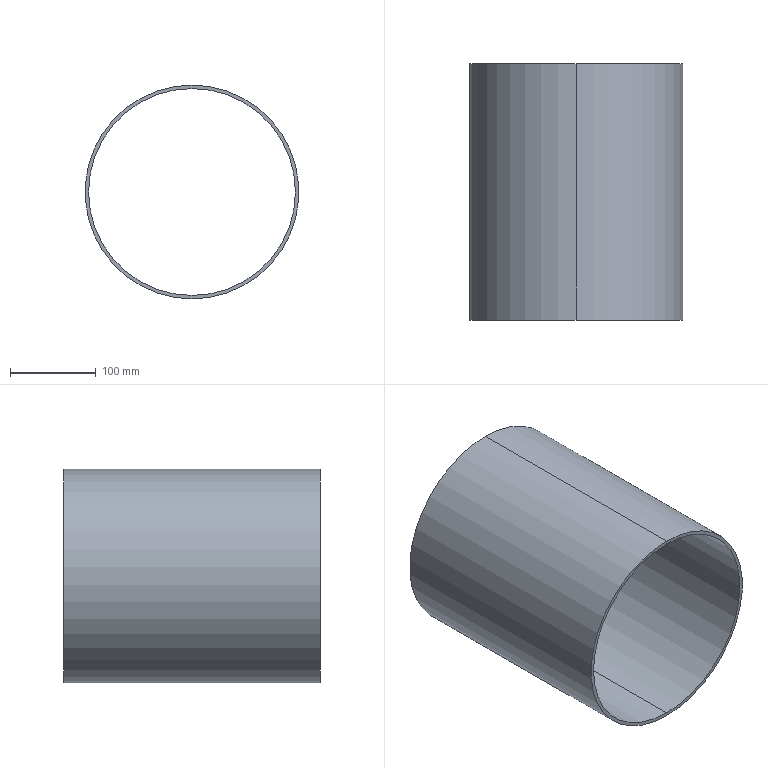Part | SolidWorks | features ExtruThin 1 | 1 solid | 6 faces | box 250 x 300 x 250 mm | volume 927398 mm3 | cylinder 4 | plane 2 | commonest cylinder face diameters 242 x2 250 x2
STEP:
#1=CARTESIAN_POINT('',(0.,300.,-121.));
#2=VERTEX_POINT('',#1);
#3=CARTESIAN_POINT('',(0.,300.,121.));
#4=VERTEX_POINT('',#3);
#5=CARTESIAN_POINT('',(0.,300.,0.));
#6=DIRECTION('',(0.,1.,0.));
#7=DIRECTION('',(1.,0.,0.));
#8=AXIS2_PLACEMENT_3D('',#5,#6,#7);
#9=CIRCLE('',#8,121.);
#10=EDGE_CURVE('',#2,#4,#9,.T.);
#11=ORIENTED_EDGE('',*,*,#10,.T.);
#12=CARTESIAN_POINT('',(0.,0.,121.));
#13=VERTEX_POINT('',#12);
#14=CARTESIAN_POINT('',(0.,300.,121.));
#15=DIRECTION('',(0.,-1.,0.));
#16=VECTOR('',#15,1000.);
#17=LINE('',#14,#16);
#18=EDGE_CURVE('',#4,#13,#17,.T.);
#19=ORIENTED_EDGE('',*,*,#18,.T.);
#20=CARTESIAN_POINT('',(0.,0.,-121.));
#21=VERTEX_POINT('',#20);
#22=CARTESIAN_POINT('',(0.,0.,0.));
#23=DIRECTION('',(0.,1.,0.));
#24=DIRECTION('',(1.,0.,0.));
#25=AXIS2_PLACEMENT_3D('',#22,#23,#24);
#26=CIRCLE('',#25,121.);
#27=EDGE_CURVE('',#21,#13,#26,.T.);
#28=ORIENTED_EDGE('',*,*,#27,.F.);
#29=CARTESIAN_POINT('',(0.,300.,-121.));
#30=DIRECTION('',(0.,-1.,0.));
#31=VECTOR('',#30,1000.);
#32=LINE('',#29,#31);
#33=EDGE_CURVE('',#2,#21,#32,.T.);
#34=ORIENTED_EDGE('',*,*,#33,.F.);
#35=EDGE_LOOP('',(#11,#19,#28,#34));
#36=FACE_OUTER_BOUND('',#35,.T.);
#37=CARTESIAN_POINT('',(0.,300.,0.));
#38=DIRECTION('',(0.,-1.,0.));
#39=DIRECTION('',(0.,0.,-1.));
#40=AXIS2_PLACEMENT_3D('',#37,#38,#39);
#41=CYLINDRICAL_SURFACE('',#40,121.);
#42=ADVANCED_FACE('',(#36),#41,.F.);
#43=CARTESIAN_POINT('',(0.,300.,125.));
#44=VERTEX_POINT('',#43);
#45=CARTESIAN_POINT('',(0.,300.,-125.));
#46=VERTEX_POINT('',#45);
#47=CARTESIAN_POINT('',(0.,300.,0.));
#48=DIRECTION('',(0.,1.,0.));
#49=DIRECTION('',(0.,0.,1.));
#50=AXIS2_PLACEMENT_3D('',#47,#48,#49);
#51=CIRCLE('',#50,125.);
#52=EDGE_CURVE('',#44,#46,#51,.T.);
#53=ORIENTED_EDGE('',*,*,#52,.F.);
#54=CARTESIAN_POINT('',(0.,0.,125.));
#55=VERTEX_POINT('',#54);
#56=CARTESIAN_POINT('',(0.,300.,125.));
#57=DIRECTION('',(0.,-1.,0.));
#58=VECTOR('',#57,1000.);
#59=LINE('',#56,#58);
#60=EDGE_CURVE('',#44,#55,#59,.T.);
#61=ORIENTED_EDGE('',*,*,#60,.T.);
#62=CARTESIAN_POINT('',(0.,0.,-125.));
#63=VERTEX_POINT('',#62);
#64=CARTESIAN_POINT('',(0.,0.,0.));
#65=DIRECTION('',(0.,1.,0.));
#66=DIRECTION('',(0.,0.,1.));
#67=AXIS2_PLACEMENT_3D('',#64,#65,#66);
#68=CIRCLE('',#67,125.);
#69=EDGE_CURVE('',#55,#63,#68,.T.);
#70=ORIENTED_EDGE('',*,*,#69,.T.);
#71=CARTESIAN_POINT('',(0.,300.,-125.));
#72=DIRECTION('',(0.,-1.,0.));
#73=VECTOR('',#72,1000.);
#74=LINE('',#71,#73);
#75=EDGE_CURVE('',#46,#63,#74,.T.);
#76=ORIENTED_EDGE('',*,*,#75,.F.);
#77=EDGE_LOOP('',(#53,#61,#70,#76));
#78=FACE_OUTER_BOUND('',#77,.T.);
#79=CARTESIAN_POINT('',(0.,300.,0.));
#80=DIRECTION('',(0.,-1.,0.));
#81=DIRECTION('',(0.,0.,-1.));
#82=AXIS2_PLACEMENT_3D('',#79,#80,#81);
#83=CYLINDRICAL_SURFACE('',#82,125.);
#84=ADVANCED_FACE('',(#78),#83,.T.);
#85=CARTESIAN_POINT('',(0.,300.,0.));
#86=DIRECTION('',(0.,1.,0.));
#87=DIRECTION('',(0.,0.,1.));
#88=AXIS2_PLACEMENT_3D('',#85,#86,#87);
#89=CIRCLE('',#88,125.);
#90=EDGE_CURVE('',#46,#44,#89,.T.);
#91=ORIENTED_EDGE('',*,*,#90,.T.);
#92=ORIENTED_EDGE('',*,*,#52,.T.);
#93=EDGE_LOOP('',(#91,#92));
#94=FACE_OUTER_BOUND('',#93,.T.);
#95=ORIENTED_EDGE('',*,*,#10,.F.);
#96=CARTESIAN_POINT('',(0.,300.,0.));
#97=DIRECTION('',(0.,1.,0.));
#98=DIRECTION('',(1.,0.,0.));
#99=AXIS2_PLACEMENT_3D('',#96,#97,#98);
#100=CIRCLE('',#99,121.);
#101=EDGE_CURVE('',#4,#2,#100,.T.);
#102=ORIENTED_EDGE('',*,*,#101,.F.);
#103=EDGE_LOOP('',(#95,#102));
#104=FACE_BOUND('',#103,.T.);
#105=CARTESIAN_POINT('',(0.,300.,0.));
#106=DIRECTION('',(0.,1.,0.));
#107=DIRECTION('',(0.,0.,1.));
#108=AXIS2_PLACEMENT_3D('',#105,#106,#107);
#109=PLANE('',#108);
#110=ADVANCED_FACE('',(#94,#104),#109,.T.);
#111=CARTESIAN_POINT('',(0.,0.,0.));
#112=DIRECTION('',(0.,1.,0.));
#113=DIRECTION('',(0.,0.,1.));
#114=AXIS2_PLACEMENT_3D('',#111,#112,#113);
#115=CIRCLE('',#114,125.);
#116=EDGE_CURVE('',#63,#55,#115,.T.);
#117=ORIENTED_EDGE('',*,*,#116,.F.);
#118=ORIENTED_EDGE('',*,*,#69,.F.);
#119=EDGE_LOOP('',(#117,#118));
#120=FACE_OUTER_BOUND('',#119,.T.);
#121=ORIENTED_EDGE('',*,*,#27,.T.);
#122=CARTESIAN_POINT('',(0.,0.,0.));
#123=DIRECTION('',(0.,1.,0.));
#124=DIRECTION('',(1.,0.,0.));
#125=AXIS2_PLACEMENT_3D('',#122,#123,#124);
#126=CIRCLE('',#125,121.);
#127=EDGE_CURVE('',#13,#21,#126,.T.);
#128=ORIENTED_EDGE('',*,*,#127,.T.);
#129=EDGE_LOOP('',(#121,#128));
#130=FACE_BOUND('',#129,.T.);
#131=CARTESIAN_POINT('',(0.,0.,0.));
#132=DIRECTION('',(0.,1.,0.));
#133=DIRECTION('',(0.,0.,1.));
#134=AXIS2_PLACEMENT_3D('',#131,#132,#133);
#135=PLANE('',#134);
#136=ADVANCED_FACE('',(#120,#130),#135,.F.);
#137=ORIENTED_EDGE('',*,*,#60,.F.);
#138=ORIENTED_EDGE('',*,*,#90,.F.);
#139=ORIENTED_EDGE('',*,*,#75,.T.);
#140=ORIENTED_EDGE('',*,*,#116,.T.);
#141=EDGE_LOOP('',(#137,#138,#139,#140));
#142=FACE_OUTER_BOUND('',#141,.T.);
#143=CARTESIAN_POINT('',(0.,300.,0.));
#144=DIRECTION('',(0.,-1.,0.));
#145=DIRECTION('',(0.,0.,-1.));
#146=AXIS2_PLACEMENT_3D('',#143,#144,#145);
#147=CYLINDRICAL_SURFACE('',#146,125.);
#148=ADVANCED_FACE('',(#142),#147,.T.);
#149=ORIENTED_EDGE('',*,*,#18,.F.);
#150=ORIENTED_EDGE('',*,*,#101,.T.);
#151=ORIENTED_EDGE('',*,*,#33,.T.);
#152=ORIENTED_EDGE('',*,*,#127,.F.);
#153=EDGE_LOOP('',(#149,#150,#151,#152));
#154=FACE_OUTER_BOUND('',#153,.T.);
#155=CARTESIAN_POINT('',(0.,300.,0.));
#156=DIRECTION('',(0.,-1.,0.));
#157=DIRECTION('',(0.,0.,-1.));
#158=AXIS2_PLACEMENT_3D('',#155,#156,#157);
#159=CYLINDRICAL_SURFACE('',#158,121.);
#160=ADVANCED_FACE('',(#154),#159,.F.);
#161=CLOSED_SHELL('',(#42,#84,#110,#136,#148,#160));
#162=MANIFOLD_SOLID_BREP('',#161);
#163=CARTESIAN_POINT('',(0.,0.,0.));
#164=DIRECTION('',(0.,0.,1.));
#165=DIRECTION('',(1.,0.,0.));
#166=AXIS2_PLACEMENT_3D('',#163,#164,#165);
#167=(LENGTH_UNIT()NAMED_UNIT(*)SI_UNIT(.MILLI.,.METRE.));
#168=UNCERTAINTY_MEASURE_WITH_UNIT(LENGTH_MEASURE(0.00001),#167,'','');
#169=(NAMED_UNIT(*)PLANE_ANGLE_UNIT()SI_UNIT($,.RADIAN.));
#170=(NAMED_UNIT(*)SI_UNIT($,.STERADIAN.)SOLID_ANGLE_UNIT());
#171=(GEOMETRIC_REPRESENTATION_CONTEXT(3)GLOBAL_UNCERTAINTY_ASSIGNED_CONTEXT((#168))GLOBAL_UNIT_ASSIGNED_CONTEXT((#167,#169,#170))REPRESENTATION_CONTEXT('',''));
#172=ADVANCED_BREP_SHAPE_REPRESENTATION('',(#162,#166),#171);